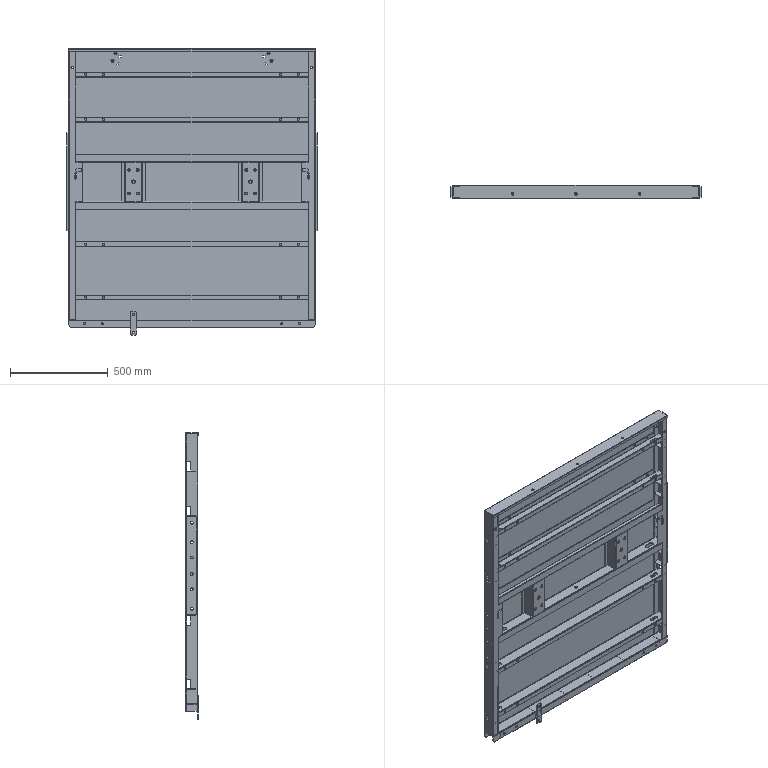Part | SolidWorks | features ReferencePattern 25, MirrorCompFeat 7, LocalLPattern 2 | 56 solids | 1610 faces | box 1280 x 70 x 1465 mm | volume 11467233 mm3 | plane 982 | cylinder 526 | cone 102 | commonest cylinder face diameters 10 x90 14.5 x88 11 x84 0.4 x36 8.4 x24 20 x24